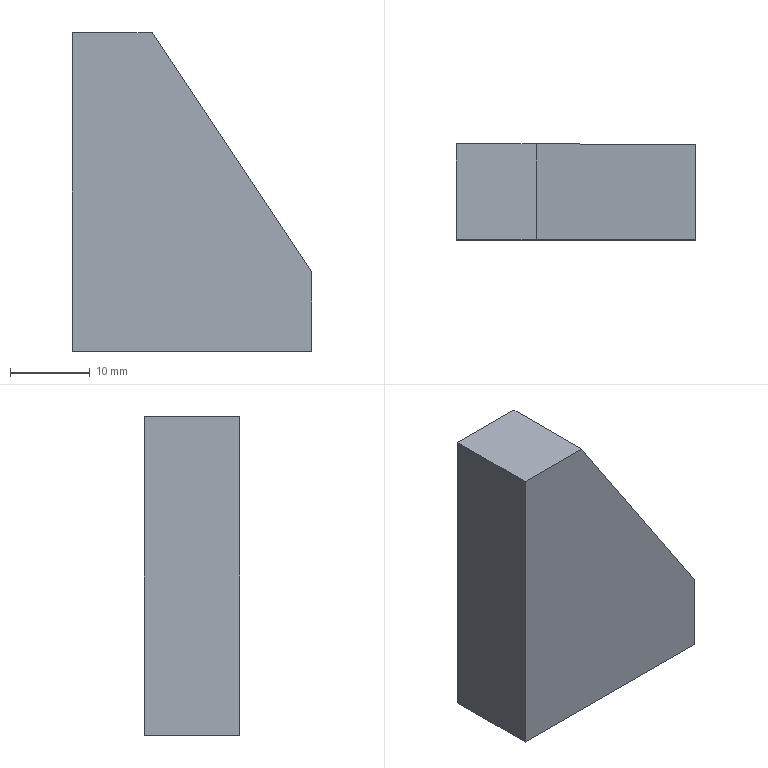Part | SolidWorks | features Extrusion 1 | 1 solid | 7 faces | box 30 x 12 x 40 mm | volume 10800 mm3 | plane 7
STEP:
#1=CARTESIAN_POINT('',(15.,-6.,-10.));
#2=VERTEX_POINT('',#1);
#3=CARTESIAN_POINT('',(15.,-6.,-20.));
#4=VERTEX_POINT('',#3);
#5=CARTESIAN_POINT('',(15.,-6.,-20.));
#6=DIRECTION('',(0.,0.,-1.));
#7=VECTOR('',#6,1000.);
#8=LINE('',#5,#7);
#9=EDGE_CURVE('',#2,#4,#8,.T.);
#10=ORIENTED_EDGE('',*,*,#9,.T.);
#11=CARTESIAN_POINT('',(15.,6.,-20.));
#12=VERTEX_POINT('',#11);
#13=CARTESIAN_POINT('',(15.,6.,-20.));
#14=DIRECTION('',(0.,-1.,0.));
#15=VECTOR('',#14,1000.);
#16=LINE('',#13,#15);
#17=EDGE_CURVE('',#12,#4,#16,.T.);
#18=ORIENTED_EDGE('',*,*,#17,.F.);
#19=CARTESIAN_POINT('',(15.,6.,-10.));
#20=VERTEX_POINT('',#19);
#21=CARTESIAN_POINT('',(15.,6.,-20.));
#22=DIRECTION('',(0.,0.,-1.));
#23=VECTOR('',#22,1000.);
#24=LINE('',#21,#23);
#25=EDGE_CURVE('',#20,#12,#24,.T.);
#26=ORIENTED_EDGE('',*,*,#25,.F.);
#27=CARTESIAN_POINT('',(15.,6.,-10.));
#28=DIRECTION('',(0.,-1.,0.));
#29=VECTOR('',#28,1000.);
#30=LINE('',#27,#29);
#31=EDGE_CURVE('',#20,#2,#30,.T.);
#32=ORIENTED_EDGE('',*,*,#31,.T.);
#33=EDGE_LOOP('',(#10,#18,#26,#32));
#34=FACE_OUTER_BOUND('',#33,.T.);
#35=CARTESIAN_POINT('',(15.,6.,-20.));
#36=DIRECTION('',(-1.,0.,0.));
#37=DIRECTION('',(0.,0.,1.));
#38=AXIS2_PLACEMENT_3D('',#35,#36,#37);
#39=PLANE('',#38);
#40=ADVANCED_FACE('',(#34),#39,.F.);
#41=CARTESIAN_POINT('',(-15.,-6.,-20.));
#42=VERTEX_POINT('',#41);
#43=CARTESIAN_POINT('',(15.,-6.,-20.));
#44=DIRECTION('',(-1.,0.,0.));
#45=VECTOR('',#44,1000.);
#46=LINE('',#43,#45);
#47=EDGE_CURVE('',#4,#42,#46,.T.);
#48=ORIENTED_EDGE('',*,*,#47,.T.);
#49=CARTESIAN_POINT('',(-15.,6.,-20.));
#50=VERTEX_POINT('',#49);
#51=CARTESIAN_POINT('',(-15.,6.,-20.));
#52=DIRECTION('',(0.,-1.,0.));
#53=VECTOR('',#52,1000.);
#54=LINE('',#51,#53);
#55=EDGE_CURVE('',#50,#42,#54,.T.);
#56=ORIENTED_EDGE('',*,*,#55,.F.);
#57=CARTESIAN_POINT('',(15.,6.,-20.));
#58=DIRECTION('',(-1.,0.,0.));
#59=VECTOR('',#58,1000.);
#60=LINE('',#57,#59);
#61=EDGE_CURVE('',#12,#50,#60,.T.);
#62=ORIENTED_EDGE('',*,*,#61,.F.);
#63=ORIENTED_EDGE('',*,*,#17,.T.);
#64=EDGE_LOOP('',(#48,#56,#62,#63));
#65=FACE_OUTER_BOUND('',#64,.T.);
#66=CARTESIAN_POINT('',(15.,6.,-20.));
#67=DIRECTION('',(0.,0.,1.));
#68=DIRECTION('',(1.,0.,0.));
#69=AXIS2_PLACEMENT_3D('',#66,#67,#68);
#70=PLANE('',#69);
#71=ADVANCED_FACE('',(#65),#70,.F.);
#72=CARTESIAN_POINT('',(-15.,-6.,20.));
#73=VERTEX_POINT('',#72);
#74=CARTESIAN_POINT('',(-15.,-6.,-20.));
#75=DIRECTION('',(0.,0.,1.));
#76=VECTOR('',#75,1000.);
#77=LINE('',#74,#76);
#78=EDGE_CURVE('',#42,#73,#77,.T.);
#79=ORIENTED_EDGE('',*,*,#78,.T.);
#80=CARTESIAN_POINT('',(-15.,6.,20.));
#81=VERTEX_POINT('',#80);
#82=CARTESIAN_POINT('',(-15.,6.,20.));
#83=DIRECTION('',(0.,-1.,0.));
#84=VECTOR('',#83,1000.);
#85=LINE('',#82,#84);
#86=EDGE_CURVE('',#81,#73,#85,.T.);
#87=ORIENTED_EDGE('',*,*,#86,.F.);
#88=CARTESIAN_POINT('',(-15.,6.,-20.));
#89=DIRECTION('',(0.,0.,1.));
#90=VECTOR('',#89,1000.);
#91=LINE('',#88,#90);
#92=EDGE_CURVE('',#50,#81,#91,.T.);
#93=ORIENTED_EDGE('',*,*,#92,.F.);
#94=ORIENTED_EDGE('',*,*,#55,.T.);
#95=EDGE_LOOP('',(#79,#87,#93,#94));
#96=FACE_OUTER_BOUND('',#95,.T.);
#97=CARTESIAN_POINT('',(-15.,6.,-20.));
#98=DIRECTION('',(1.,0.,0.));
#99=DIRECTION('',(0.,0.,-1.));
#100=AXIS2_PLACEMENT_3D('',#97,#98,#99);
#101=PLANE('',#100);
#102=ADVANCED_FACE('',(#96),#101,.F.);
#103=CARTESIAN_POINT('',(-5.,-6.,20.));
#104=VERTEX_POINT('',#103);
#105=CARTESIAN_POINT('',(-15.,-6.,20.));
#106=DIRECTION('',(1.,0.,0.));
#107=VECTOR('',#106,1000.);
#108=LINE('',#105,#107);
#109=EDGE_CURVE('',#73,#104,#108,.T.);
#110=ORIENTED_EDGE('',*,*,#109,.T.);
#111=CARTESIAN_POINT('',(-5.,6.,20.));
#112=VERTEX_POINT('',#111);
#113=CARTESIAN_POINT('',(-5.,6.,20.));
#114=DIRECTION('',(0.,-1.,0.));
#115=VECTOR('',#114,1000.);
#116=LINE('',#113,#115);
#117=EDGE_CURVE('',#112,#104,#116,.T.);
#118=ORIENTED_EDGE('',*,*,#117,.F.);
#119=CARTESIAN_POINT('',(-15.,6.,20.));
#120=DIRECTION('',(1.,0.,0.));
#121=VECTOR('',#120,1000.);
#122=LINE('',#119,#121);
#123=EDGE_CURVE('',#81,#112,#122,.T.);
#124=ORIENTED_EDGE('',*,*,#123,.F.);
#125=ORIENTED_EDGE('',*,*,#86,.T.);
#126=EDGE_LOOP('',(#110,#118,#124,#125));
#127=FACE_OUTER_BOUND('',#126,.T.);
#128=CARTESIAN_POINT('',(-15.,6.,20.));
#129=DIRECTION('',(0.,0.,-1.));
#130=DIRECTION('',(-1.,0.,0.));
#131=AXIS2_PLACEMENT_3D('',#128,#129,#130);
#132=PLANE('',#131);
#133=ADVANCED_FACE('',(#127),#132,.F.);
#134=CARTESIAN_POINT('',(15.,-6.,-10.));
#135=DIRECTION('',(0.5547,0.,-0.8321));
#136=VECTOR('',#135,1000.);
#137=LINE('',#134,#136);
#138=EDGE_CURVE('',#104,#2,#137,.T.);
#139=ORIENTED_EDGE('',*,*,#138,.T.);
#140=ORIENTED_EDGE('',*,*,#31,.F.);
#141=CARTESIAN_POINT('',(15.,6.,-10.));
#142=DIRECTION('',(0.5547,0.,-0.8321));
#143=VECTOR('',#142,1000.);
#144=LINE('',#141,#143);
#145=EDGE_CURVE('',#112,#20,#144,.T.);
#146=ORIENTED_EDGE('',*,*,#145,.F.);
#147=ORIENTED_EDGE('',*,*,#117,.T.);
#148=EDGE_LOOP('',(#139,#140,#146,#147));
#149=FACE_OUTER_BOUND('',#148,.T.);
#150=CARTESIAN_POINT('',(15.,6.,-10.));
#151=DIRECTION('',(-0.8321,0.,-0.5547));
#152=DIRECTION('',(-0.5547,0.,0.8321));
#153=AXIS2_PLACEMENT_3D('',#150,#151,#152);
#154=PLANE('',#153);
#155=ADVANCED_FACE('',(#149),#154,.F.);
#156=ORIENTED_EDGE('',*,*,#25,.T.);
#157=ORIENTED_EDGE('',*,*,#61,.T.);
#158=ORIENTED_EDGE('',*,*,#92,.T.);
#159=ORIENTED_EDGE('',*,*,#123,.T.);
#160=ORIENTED_EDGE('',*,*,#145,.T.);
#161=EDGE_LOOP('',(#156,#157,#158,#159,#160));
#162=FACE_OUTER_BOUND('',#161,.T.);
#163=CARTESIAN_POINT('',(15.,6.,20.));
#164=DIRECTION('',(0.,1.,0.));
#165=DIRECTION('',(0.,0.,1.));
#166=AXIS2_PLACEMENT_3D('',#163,#164,#165);
#167=PLANE('',#166);
#168=ADVANCED_FACE('',(#162),#167,.T.);
#169=ORIENTED_EDGE('',*,*,#9,.F.);
#170=ORIENTED_EDGE('',*,*,#138,.F.);
#171=ORIENTED_EDGE('',*,*,#109,.F.);
#172=ORIENTED_EDGE('',*,*,#78,.F.);
#173=ORIENTED_EDGE('',*,*,#47,.F.);
#174=EDGE_LOOP('',(#169,#170,#171,#172,#173));
#175=FACE_OUTER_BOUND('',#174,.T.);
#176=CARTESIAN_POINT('',(15.,-6.,20.));
#177=DIRECTION('',(0.,1.,0.));
#178=DIRECTION('',(0.,0.,1.));
#179=AXIS2_PLACEMENT_3D('',#176,#177,#178);
#180=PLANE('',#179);
#181=ADVANCED_FACE('',(#175),#180,.F.);
#182=CLOSED_SHELL('',(#40,#71,#102,#133,#155,#168,#181));
#183=MANIFOLD_SOLID_BREP('',#182);
#184=CARTESIAN_POINT('',(0.,0.,0.));
#185=DIRECTION('',(0.,0.,1.));
#186=DIRECTION('',(1.,0.,0.));
#187=AXIS2_PLACEMENT_3D('',#184,#185,#186);
#188=(LENGTH_UNIT()NAMED_UNIT(*)SI_UNIT(.MILLI.,.METRE.));
#189=UNCERTAINTY_MEASURE_WITH_UNIT(LENGTH_MEASURE(0.00001),#188,'','');
#190=(NAMED_UNIT(*)PLANE_ANGLE_UNIT()SI_UNIT($,.RADIAN.));
#191=(NAMED_UNIT(*)SI_UNIT($,.STERADIAN.)SOLID_ANGLE_UNIT());
#192=(GEOMETRIC_REPRESENTATION_CONTEXT(3)GLOBAL_UNCERTAINTY_ASSIGNED_CONTEXT((#189))GLOBAL_UNIT_ASSIGNED_CONTEXT((#188,#190,#191))REPRESENTATION_CONTEXT('',''));
#193=ADVANCED_BREP_SHAPE_REPRESENTATION('',(#183,#187),#192);